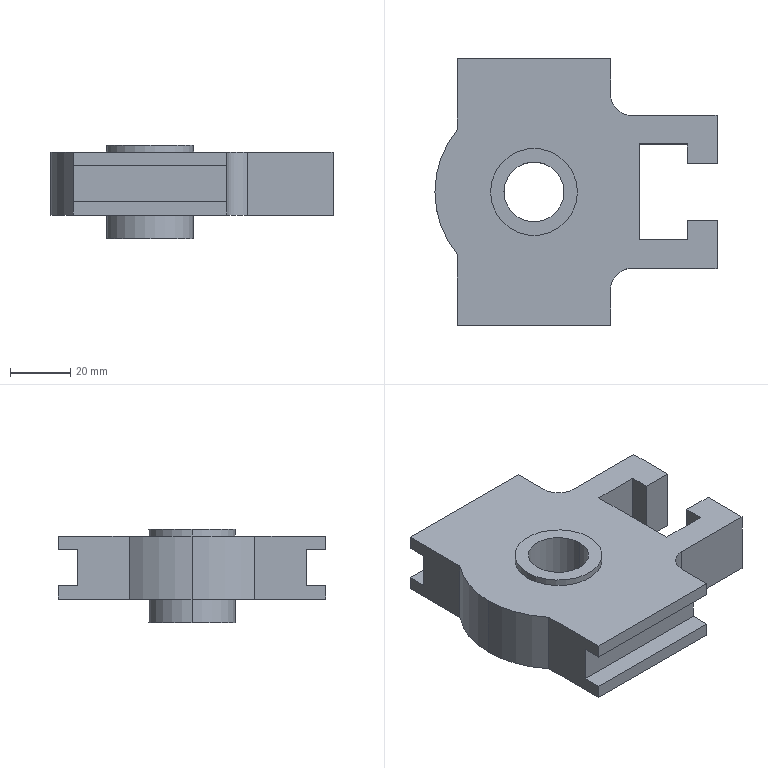Part | STEP file | UCT204 | 1 solid | 39 faces | box 94 x 89 x 31 mm | volume 112461 mm3 | plane 29 | cylinder 10 | commonest cylinder face diameters 29 x4 14.03 x2 20 x2 66 x2